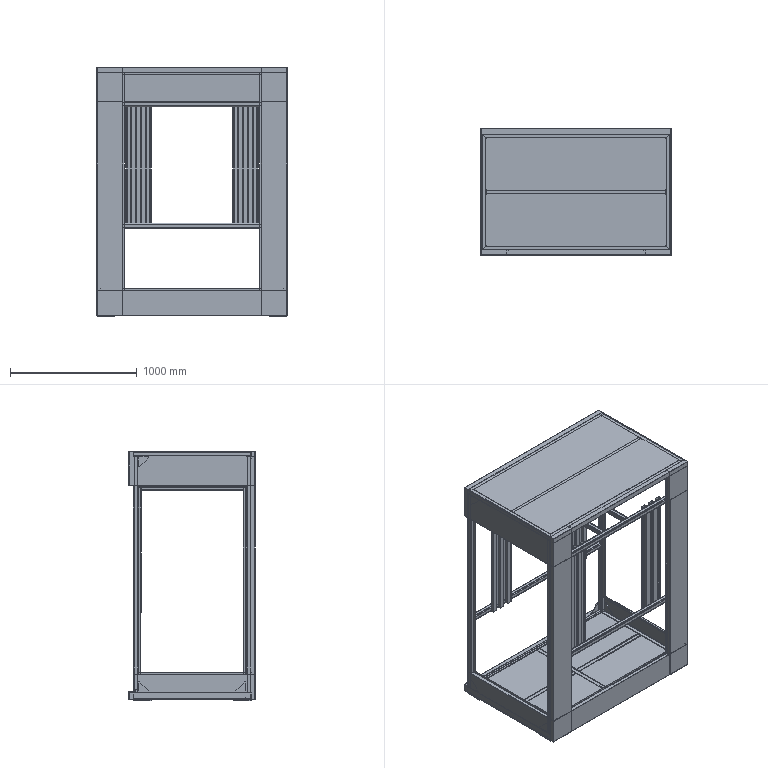Part | SolidWorks | 61 solids | 1506 faces | box 1502 x 997.4 x 1969 mm | volume 40879117 mm3 | plane 1118 | cylinder 388 | commonest cylinder face diameters 2 x100 8 x72 4.4 x62 16 x60 4 x38 6.4 x28